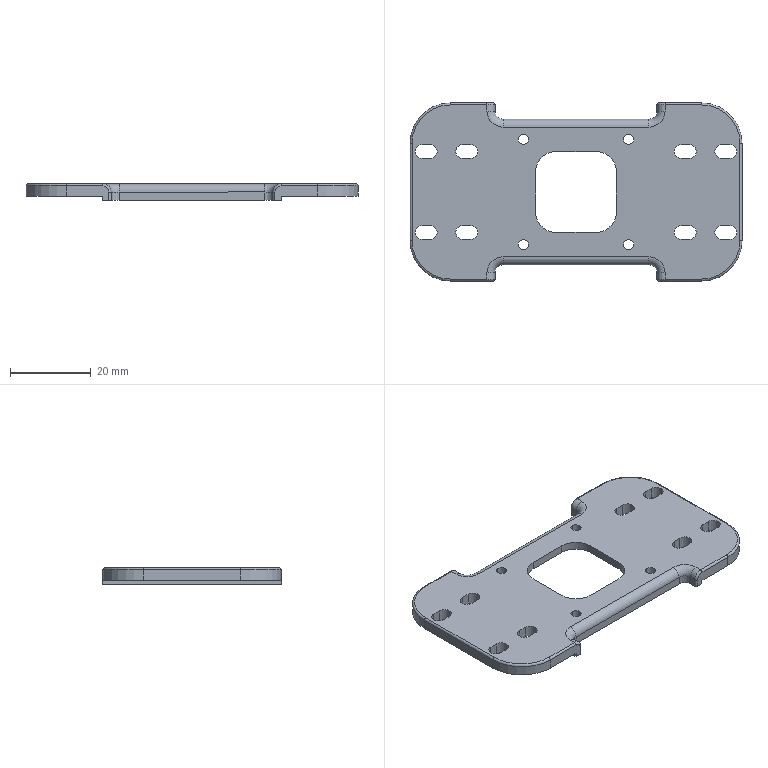NC program | NX | posted with a generic post | part box 82 x 44 x 4 mm
Lines 732 to 1673 of 6362:
(ZLEVEL_PROFILE_COPY_1 , TOOL : D3)
N1432 T16 M6
N1434 G54
N1436 G17 G0 G90 X-19.135 Y22.56 S9500 M3
N1438 G43 Z30. H16
N1440 Z1.214
N1442 G94 G1 Z-0.286 F1000.
N1444 X-19.461 Y22.23
N1446 G3 X-19.537 Y21.94 R0.3
N1448 G2 X-19.47 Y21.5 R1.938 F1200.
N1450 G1 Y20.
N1452 G3 X-18. Y18.53 R1.47
N1454 G1 X-15.874
N1456 G3 X-15.614 Y18.68 R0.3
N1458 G1 X-15.354 Y19.13
N1460 Z1.214
N1462 G0 X-18.813 Y22.683 Z0.929
N1464 G1 Z-0.571 F1000.
N1466 X-19.127 Y22.34
N1468 G3 X-19.191 Y22.047 R0.3
N1470 G2 X-19.1 Y21.5 R1.975 F1200.
N1472 G1 Y20.
N1474 G3 X-18. Y18.9 R1.1
N1476 G1 X-15.569
N1478 G3 X-15.31 Y19.05 R0.3
N1480 G1 X-15.05 Y19.5
N1482 Z0.929
N1484 G0 X-18.644 Y22.827 Z0.643
N1486 G1 Z-0.857 F1000.
N1488 X-18.939 Y22.468
N1490 G3 X-18.987 Y22.171 R0.3
N1492 G2 X-18.859 Y21.5 R1.996 F1200.
N1494 G1 Y20.
N1496 G3 X-18. Y19.141 R0.859
N1498 G1 X-15.358
N1500 G3 X-15.098 Y19.291 R0.3
N1502 G1 X-14.838 Y19.741
N1504 Z0.643
N1506 G0 X-18.512 Y22.893 Z0.357
N1508 G1 Z-1.143 F1000.
N1510 X-18.798 Y22.526
N1512 G3 X-18.84 Y22.229 R0.3
N1514 G2 X-18.693 Y21.5 R2.014 F1200.
N1516 G1 Y20.
N1518 G3 X-18. Y19.307 R0.693
N1520 G1 X-15.23
N1522 G3 X-14.97 Y19.457 R0.3
N1524 G1 X-14.71 Y19.907
N1526 Z0.357
N1528 G0 X-18.421 Y22.93 Z0.071
N1530 G1 Z-1.429 F1000.
N1532 X-18.703 Y22.559
N1534 G3 X-18.741 Y22.262 R0.3
N1536 G2 X-18.583 Y21.5 R2.021 F1200.
N1538 G1 Y20.
N1540 G3 X-18. Y19.417 R0.583
N1542 G1 X-15.149
N1544 G3 X-14.889 Y19.567 R0.3
N1546 G1 X-14.629 Y20.017
N1548 Z0.071
N1550 G0 X-18.396 Y22.989 Z-0.214
N1552 G1 Z-1.714 F1000.
N1554 X-18.668 Y22.611
N1556 G3 X-18.698 Y22.313 R0.3
N1558 G2 X-18.564 Y21.901 R2.015 F1200.
N1560 G1 X-18.521 Y21.5
N1562 Y20.
N1564 G3 X-18. Y19.479 R0.521
N1566 G1 X-15.103
N1568 G3 X-14.843 Y19.629 R0.3
N1570 G1 X-14.583 Y20.079
N1572 Z-0.214
N1574 G0 X-18.361 Y22.977 Z-0.5
N1576 G1 Z-2. F1000.
N1578 X-18.637 Y22.603
N1580 G3 X-18.67 Y22.304 R0.3
N1582 G2 X-18.503 Y21.542 R1.997 F1200.
N1584 G1 X-18.5 Y21.297
N1586 Y20.
N1588 G3 X-18. Y19.5 R0.5
N1590 G1 X-15.098
N1592 G3 X-14.839 Y19.65 R0.3
N1594 G1 X-14.579 Y20.1
N1596 Z-0.5
N1598 G0 X-18.361 Y22.977 Z-0.786
N1600 G1 Z-2.286 F1000.
N1602 X-18.636 Y22.602
N1604 G3 X-18.669 Y22.304 R0.3
N1606 G2 X-18.5 Y21.5 R2. F1200.
N1608 G1 Y20.
N1610 G3 X-18. Y19.5 R0.5
N1612 G1 X-15.083
N1614 G3 X-14.823 Y19.65 R0.3
N1616 G1 X-14.564 Y20.1
N1618 Z-0.786
N1620 G0 X-18.361 Y22.977 Z-1.071
N1622 G1 Z-2.571 F1000.
N1624 X-18.636 Y22.602
N1626 G3 X-18.669 Y22.304 R0.3
N1628 G2 X-18.5 Y21.5 R2. F1200.
N1630 G1 Y20.
N1632 G3 X-18. Y19.5 R0.5
N1634 G1 X-15.083
N1636 G3 X-14.823 Y19.65 R0.3
N1638 G1 X-14.564 Y20.1
N1640 Z-1.071
N1642 G0 X-18.361 Y22.977 Z-1.357
N1644 G1 Z-2.857 F1000.
N1646 X-18.636 Y22.602
N1648 G3 X-18.669 Y22.304 R0.3
N1650 G2 X-18.5 Y21.5 R2. F1200.
N1652 G1 Y20.
N1654 G3 X-18. Y19.5 R0.5
N1656 G1 X-15.083
N1658 G3 X-14.823 Y19.65 R0.3
N1660 G1 X-14.564 Y20.1
N1662 Z-1.357
N1664 G0 X-18.361 Y22.977 Z-1.643
N1666 G1 Z-3.143 F1000.
N1668 X-18.636 Y22.602
N1670 G3 X-18.669 Y22.304 R0.3
N1672 G2 X-18.5 Y21.5 R2. F1200.
N1674 G1 Y20.
N1676 G3 X-18. Y19.5 R0.5
N1678 G1 X-15.083
N1680 G3 X-14.823 Y19.65 R0.3
N1682 G1 X-14.564 Y20.1
N1684 Z-1.643
N1686 G0 X-18.361 Y22.977 Z-1.929
N1688 G1 Z-3.429 F1000.
N1690 X-18.636 Y22.602
N1692 G3 X-18.669 Y22.304 R0.3
N1694 G2 X-18.5 Y21.5 R2. F1200.
N1696 G1 Y20.
N1698 G3 X-18. Y19.5 R0.5
N1700 G1 X-15.083
N1702 G3 X-14.823 Y19.65 R0.3
N1704 G1 X-14.564 Y20.1
N1706 Z-1.929
N1708 G0 X-18.361 Y22.977 Z-2.214
N1710 G1 Z-3.714 F1000.
N1712 X-18.636 Y22.602
N1714 G3 X-18.669 Y22.304 R0.3
N1716 G2 X-18.5 Y21.5 R2. F1200.
N1718 G1 Y20.
N1720 G3 X-18. Y19.5 R0.5
N1722 G1 X-15.083
N1724 G3 X-14.823 Y19.65 R0.3
N1726 G1 X-14.564 Y20.1
N1728 Z-2.214
N1730 G0 X-18.361 Y22.977 Z-2.5
N1732 G1 Z-4. F1000.
N1734 X-18.636 Y22.602
N1736 G3 X-18.669 Y22.304 R0.3
N1738 G2 X-18.5 Y21.5 R2. F1200.
N1740 G1 Y20.
N1742 G3 X-18. Y19.5 R0.5
N1744 G1 X-15.083
N1746 G3 X-14.823 Y19.65 R0.3
N1748 G1 X-14.564 Y20.1
N1750 Z-2.5
N1752 G0 Z30.
N1754 X15.354 Y19.13
N1756 Z1.214
N1758 G1 Z-0.286 F1000.
N1760 X15.614 Y18.68
N1762 G3 X15.874 Y18.53 R0.3
N1764 G1 X18. F1200.
N1766 G3 X19.47 Y20. R1.47
N1768 G1 Y21.5
N1770 G2 X19.538 Y21.94 R1.938
N1772 G3 X19.462 Y22.231 R0.3
N1774 G1 X19.135 Y22.561
N1776 Z1.214
N1778 G0 X15.04 Y19.5 Z0.929
N1780 G1 Z-0.571 F1000.
N1782 X15.3 Y19.05
N1784 G3 X15.56 Y18.9 R0.3
N1786 G1 X18. F1200.
N1788 G3 X19.1 Y20. R1.1
N1790 G1 Y21.5
N1792 G2 X19.192 Y22.047 R1.975
N1794 G3 X19.127 Y22.34 R0.3
N1796 G1 X18.813 Y22.683
N1798 Z0.929
N1800 G0 X14.842 Y19.741 Z0.643
N1802 G1 Z-0.857 F1000.
N1804 X15.102 Y19.291
N1806 G3 X15.362 Y19.141 R0.3
N1808 G1 X18. F1200.
N1810 G3 X18.859 Y20. R0.859
N1812 G1 Y21.5
N1814 G2 X18.986 Y22.168 R1.996
N1816 G3 X18.937 Y22.464 R0.3
N1818 G1 X18.641 Y22.823
N1820 Z0.643
N1822 G0 X14.711 Y19.907 Z0.357
N1824 G1 Z-1.143 F1000.
N1826 X14.971 Y19.457
N1828 G3 X15.231 Y19.307 R0.3
N1830 G1 X18. F1200.
N1832 G3 X18.693 Y20. R0.693
N1834 G1 Y21.5
N1836 G2 X18.838 Y22.225 R2.013
N1838 G3 X18.796 Y22.522 R0.3
N1840 G1 X18.508 Y22.888
N1842 Z0.357
N1844 G0 X14.64 Y20.017 Z0.071
N1846 G1 Z-1.429 F1000.
N1848 X14.9 Y19.567
N1850 G3 X15.16 Y19.417 R0.3
N1852 G1 X18. F1200.
N1854 G3 X18.583 Y20. R0.583
N1856 G1 Y21.5
N1858 G2 X18.742 Y22.265 R2.021
N1860 G3 X18.705 Y22.563 R0.3
N1862 G1 X18.424 Y22.934
N1864 Z0.071
N1866 G0 X14.582 Y20.079 Z-0.214
N1868 G1 Z-1.714 F1000.
N1870 X14.842 Y19.629
N1872 G3 X15.102 Y19.479 R0.3
N1874 G1 X18. F1200.
N1876 G3 X18.521 Y20. R0.521
N1878 G1 Y21.5
N1880 G2 X18.698 Y22.307 R2.16
N1882 G3 X18.663 Y22.605 R0.3
N1884 G1 X18.386 Y22.978
N1886 Z-0.214
N1888 G0 X14.579 Y20.1 Z-0.5
N1890 G1 Z-2. F1000.
N1892 X14.839 Y19.65
N1894 G3 X15.098 Y19.5 R0.3
N1896 G1 X18. F1200.
N1898 G3 X18.5 Y20. R0.499
N1900 G1 X18.501 Y20.073
N1902 Y21.297
N1904 X18.503 Y21.542
N1906 G2 X18.671 Y22.305 R1.998
N1908 G3 X18.638 Y22.603 R0.3
N1910 G1 X18.363 Y22.978
N1912 Z-0.5
N1914 G0 X14.564 Y20.1 Z-0.786
N1916 G1 Z-2.286 F1000.
N1918 X14.823 Y19.65
N1920 G3 X15.083 Y19.5 R0.3
N1922 G1 X18. F1200.
N1924 G3 X18.5 Y20. R0.5
N1926 G1 Y21.5
N1928 X18.507 Y21.649
N1930 X18.506
N1932 G2 X18.669 Y22.304 R2.
N1934 G3 X18.636 Y22.602 R0.3
N1936 G1 X18.361 Y22.977
N1938 Z-0.786
N1940 G0 X14.564 Y20.1 Z-1.071
N1942 G1 Z-2.571 F1000.
N1944 X14.823 Y19.65
N1946 G3 X15.083 Y19.5 R0.3
N1948 G1 X18. F1200.
N1950 G3 X18.5 Y20. R0.5
N1952 G1 Y21.5
N1954 X18.507 Y21.649
N1956 X18.506
N1958 G2 X18.669 Y22.304 R2.
N1960 G3 X18.636 Y22.602 R0.3
N1962 G1 X18.361 Y22.977
N1964 Z-1.071
N1966 G0 X14.564 Y20.1 Z-1.357
N1968 G1 Z-2.857 F1000.
N1970 X14.823 Y19.65
N1972 G3 X15.083 Y19.5 R0.3
N1974 G1 X18. F1200.
N1976 G3 X18.5 Y20. R0.5
N1978 G1 Y21.5
N1980 X18.507 Y21.649
N1982 X18.506
N1984 G2 X18.669 Y22.304 R2.
N1986 G3 X18.636 Y22.602 R0.3
N1988 G1 X18.361 Y22.977
N1990 Z-1.357
N1992 G0 X14.564 Y20.1 Z-1.643
N1994 G1 Z-3.143 F1000.
N1996 X14.823 Y19.65
N1998 G3 X15.083 Y19.5 R0.3
N2000 G1 X18. F1200.
N2002 G3 X18.5 Y20. R0.5
N2004 G1 Y21.5
N2006 X18.507 Y21.649
N2008 X18.506
N2010 G2 X18.669 Y22.304 R2.
N2012 G3 X18.636 Y22.602 R0.3
N2014 G1 X18.361 Y22.977
N2016 Z-1.643
N2018 G0 X14.564 Y20.1 Z-1.929
N2020 G1 Z-3.429 F1000.
N2022 X14.823 Y19.65
N2024 G3 X15.083 Y19.5 R0.3
N2026 G1 X18. F1200.
N2028 G3 X18.5 Y20. R0.5
N2030 G1 Y21.5
N2032 X18.507 Y21.649
N2034 X18.506
N2036 G2 X18.669 Y22.304 R2.
N2038 G3 X18.636 Y22.602 R0.3
N2040 G1 X18.361 Y22.977
N2042 Z-1.929
N2044 G0 X14.564 Y20.1 Z-2.214
N2046 G1 Z-3.714 F1000.
N2048 X14.823 Y19.65
N2050 G3 X15.083 Y19.5 R0.3
N2052 G1 X18. F1200.
N2054 G3 X18.5 Y20. R0.5
N2056 G1 Y21.5
N2058 X18.507 Y21.649
N2060 X18.506
N2062 G2 X18.669 Y22.304 R2.
N2064 G3 X18.636 Y22.602 R0.3
N2066 G1 X18.361 Y22.977
N2068 Z-2.214
N2070 G0 X14.564 Y20.1 Z-2.5
N2072 G1 Z-4. F1000.
N2074 X14.823 Y19.65
N2076 G3 X15.083 Y19.5 R0.3
N2078 G1 X18. F1200.
N2080 G3 X18.5 Y20. R0.5
N2082 G1 Y21.5
N2084 X18.507 Y21.649
N2086 X18.506
N2088 G2 X18.669 Y22.304 R2.
N2090 G3 X18.636 Y22.602 R0.3
N2092 G1 X18.361 Y22.977
N2094 Z-2.5
N2096 G0 Z30.
N2098 X19.135 Y-22.561
N2100 Z1.214
N2102 G1 Z-0.286 F1000.
N2104 X19.462 Y-22.231
N2106 G3 X19.538 Y-21.94 R0.3
N2108 G2 X19.47 Y-21.5 R1.938 F1200.
N2110 G1 Y-20.
N2112 G3 X18. Y-18.53 R1.47
N2114 G1 X15.874
N2116 G3 X15.614 Y-18.68 R0.3
N2118 G1 X15.354 Y-19.13
N2120 Z1.214
N2122 G0 X18.813 Y-22.683 Z0.929
N2124 G1 Z-0.571 F1000.
N2126 X19.127 Y-22.34
N2128 G3 X19.191 Y-22.047 R0.3
N2130 G2 X19.1 Y-21.5 R1.975 F1200.
N2132 G1 Y-20.
N2134 G3 X18. Y-18.9 R1.1
N2136 G1 X15.569
N2138 G3 X15.31 Y-19.05 R0.3
N2140 G1 X15.05 Y-19.5
N2142 Z0.929
N2144 G0 X18.642 Y-22.825 Z0.643
N2146 G1 Z-0.857 F1000.
N2148 X18.937 Y-22.465
N2150 G3 X18.985 Y-22.169 R0.3
N2152 G2 X18.859 Y-21.5 R1.982 F1200.
N2154 G1 Y-20.
N2156 G3 X18. Y-19.141 R0.859
N2158 G1 X15.358
N2160 G3 X15.098 Y-19.291 R0.3
N2162 G1 X14.838 Y-19.741
N2164 Z0.643
N2166 G0 X18.51 Y-22.891 Z0.357
N2168 G1 Z-1.143 F1000.
N2170 X18.797 Y-22.525
N2172 G3 X18.839 Y-22.228 R0.3
N2174 G2 X18.693 Y-21.5 R2.01 F1200.
N2176 G1 Y-20.
N2178 G3 X18. Y-19.307 R0.693
N2180 G1 X15.23
N2182 G3 X14.97 Y-19.457 R0.3
N2184 G1 X14.71 Y-19.907
N2186 Z0.357
N2188 G0 X18.422 Y-22.93 Z0.071
N2190 G1 Z-1.429 F1000.
N2192 X18.703 Y-22.559
N2194 G3 X18.741 Y-22.262 R0.3
N2196 G2 X18.583 Y-21.5 R2.021 F1200.
N2198 G1 Y-20.
N2200 G3 X18. Y-19.417 R0.583
N2202 G1 X15.149
N2204 G3 X14.889 Y-19.567 R0.3
N2206 G1 X14.629 Y-20.017
N2208 Z0.071
N2210 G0 X18.385 Y-22.972 Z-0.214
N2212 G1 Z-1.714 F1000.
N2214 X18.659 Y-22.596
N2216 G3 X18.692 Y-22.298 R0.3
N2218 G2 X18.564 Y-21.901 R2.015 F1200.
N2220 X18.521 Y-21.5 R3.783
N2222 G1 Y-20.
N2224 G3 X18. Y-19.479 R0.521
N2226 G1 X15.103
N2228 G3 X14.843 Y-19.629 R0.3
N2230 G1 X14.583 Y-20.079
N2232 Z-0.214
N2234 G0 X18.358 Y-22.97 Z-0.5
N2236 G1 Z-2. F1000.
N2238 X18.634 Y-22.596
N2240 G3 X18.668 Y-22.298 R0.3
N2242 G2 X18.501 Y-21.5 R2.002 F1200.
N2244 G1 Y-20.
N2246 G3 X18. Y-19.499 R0.501
N2248 G1 X15.091
N2250 G3 X14.831 Y-19.649 R0.3
N2252 G1 X14.572 Y-20.099
N2254 Z-0.5
N2256 G0 X18.361 Y-22.977 Z-0.786
N2258 G1 Z-2.286 F1000.
N2260 X18.636 Y-22.602
N2262 G3 X18.669 Y-22.304 R0.3
N2264 G2 X18.5 Y-21.5 R2. F1200.
N2266 G1 Y-20.
N2268 G3 X18. Y-19.5 R0.5
N2270 G1 X15.083
N2272 G3 X14.823 Y-19.65 R0.3
N2274 G1 X14.564 Y-20.1
N2276 Z-0.786
N2278 G0 X18.361 Y-22.977 Z-1.071
N2280 G1 Z-2.571 F1000.
N2282 X18.636 Y-22.602
N2284 G3 X18.669 Y-22.304 R0.3
N2286 G2 X18.5 Y-21.5 R2. F1200.
N2288 G1 Y-20.
N2290 G3 X18. Y-19.5 R0.5
N2292 G1 X15.083
N2294 G3 X14.823 Y-19.65 R0.3
N2296 G1 X14.564 Y-20.1
N2298 Z-1.071
N2300 G0 X18.361 Y-22.977 Z-1.357
N2302 G1 Z-2.857 F1000.
N2304 X18.636 Y-22.602
N2306 G3 X18.669 Y-22.304 R0.3
N2308 G2 X18.5 Y-21.5 R2. F1200.
N2310 G1 Y-20.
N2312 G3 X18. Y-19.5 R0.5
N2314 G1 X15.083
N2316 G3 X14.823 Y-19.65 R0.3
N2318 G1 X14.564 Y-20.1
N2320 Z-1.357
N2322 G0 X18.361 Y-22.977 Z-1.643
N2324 G1 Z-3.143 F1000.
N2326 X18.636 Y-22.602
N2328 G3 X18.669 Y-22.304 R0.3
N2330 G2 X18.5 Y-21.5 R2. F1200.
N2332 G1 Y-20.
N2334 G3 X18. Y-19.5 R0.5
N2336 G1 X15.083
N2338 G3 X14.823 Y-19.65 R0.3
N2340 G1 X14.564 Y-20.1
N2342 Z-1.643
N2344 G0 X18.361 Y-22.977 Z-1.929
N2346 G1 Z-3.429 F1000.
N2348 X18.636 Y-22.602
N2350 G3 X18.669 Y-22.304 R0.3
N2352 G2 X18.5 Y-21.5 R2. F1200.
N2354 G1 Y-20.
N2356 G3 X18. Y-19.5 R0.5
N2358 G1 X15.083
N2360 G3 X14.823 Y-19.65 R0.3
N2362 G1 X14.564 Y-20.1
N2364 Z-1.929
N2366 G0 X18.361 Y-22.977 Z-2.214
N2368 G1 Z-3.714 F1000.
N2370 X18.636 Y-22.602
N2372 G3 X18.669 Y-22.304 R0.3
N2374 G2 X18.5 Y-21.5 R2. F1200.
N2376 G1 Y-20.
N2378 G3 X18. Y-19.5 R0.5
N2380 G1 X15.083
N2382 G3 X14.823 Y-19.65 R0.3
N2384 G1 X14.564 Y-20.1
N2386 Z-2.214
N2388 G0 X18.361 Y-22.977 Z-2.5
N2390 G1 Z-4. F1000.
N2392 X18.636 Y-22.602
N2394 G3 X18.669 Y-22.304 R0.3
N2396 G2 X18.5 Y-21.5 R2. F1200.
N2398 G1 Y-20.
N2400 G3 X18. Y-19.5 R0.5
N2402 G1 X15.083
N2404 G3 X14.823 Y-19.65 R0.3
N2406 G1 X14.564 Y-20.1
N2408 Z-2.5
N2410 G0 Z30.
N2412 X-15.354 Y-19.13
N2414 Z1.214
N2416 G1 Z-0.286 F1000.
N2418 X-15.614 Y-18.68
N2420 G3 X-15.874 Y-18.53 R0.3
N2422 G1 X-18. F1200.
N2424 G3 X-19.47 Y-20. R1.47
N2426 G1 Y-21.5
N2428 G2 X-19.537 Y-21.94 R1.938
N2430 G3 X-19.462 Y-22.23 R0.3
N2432 G1 X-19.135 Y-22.561
N2434 Z1.214
N2436 G0 X-15.04 Y-19.5 Z0.929
N2438 G1 Z-0.571 F1000.
N2440 X-15.3 Y-19.05
N2442 G3 X-15.56 Y-18.9 R0.3
N2444 G1 X-18. F1200.
N2446 G3 X-19.1 Y-20. R1.1
N2448 G1 Y-21.5
N2450 G2 X-19.192 Y-22.047 R1.975
N2452 G3 X-19.127 Y-22.34 R0.3
N2454 G1 X-18.813 Y-22.683
N2456 Z0.929
N2458 G0 X-14.842 Y-19.741 Z0.643
N2460 G1 Z-0.857 F1000.
N2462 X-15.102 Y-19.291
N2464 G3 X-15.362 Y-19.141 R0.3
N2466 G1 X-18. F1200.
N2468 G3 X-18.859 Y-20. R0.859
N2470 G1 Y-21.5
N2472 G2 X-18.986 Y-22.168 R1.996
N2474 G3 X-18.937 Y-22.464 R0.3
N2476 G1 X-18.641 Y-22.823
N2478 Z0.643
N2480 G0 X-14.711 Y-19.907 Z0.357
N2482 G1 Z-1.143 F1000.
N2484 X-14.971 Y-19.457
N2486 G3 X-15.231 Y-19.307 R0.3
N2488 G1 X-18. F1200.
N2490 G3 X-18.693 Y-20. R0.693
N2492 G1 Y-21.5
N2494 G2 X-18.838 Y-22.225 R2.013
N2496 G3 X-18.796 Y-22.522 R0.3
N2498 G1 X-18.508 Y-22.888
N2500 Z0.357
N2502 G0 X-14.64 Y-20.017 Z0.071
N2504 G1 Z-1.429 F1000.
N2506 X-14.9 Y-19.567
N2508 G3 X-15.16 Y-19.417 R0.3
N2510 G1 X-18. F1200.
N2512 G3 X-18.583 Y-20. R0.583
N2514 G1 Y-21.5
N2516 G2 X-18.742 Y-22.265 R2.021
N2518 G3 X-18.705 Y-22.563 R0.3
N2520 G1 X-18.424 Y-22.934
N2522 Z0.071
N2524 G0 X-14.583 Y-20.079 Z-0.214
N2526 G1 Z-1.714 F1000.
N2528 X-14.842 Y-19.629
N2530 G3 X-15.102 Y-19.479 R0.3
N2532 G1 X-18. F1200.
N2534 G3 X-18.521 Y-20. R0.521
N2536 G1 Y-21.5
N2538 G2 X-18.696 Y-22.304 R2.152
N2540 G3 X-18.662 Y-22.602 R0.3
N2542 G1 X-18.385 Y-22.975
N2544 Z-0.214
N2546 G0 X-14.569 Y-20.099 Z-0.5
N2548 G1 Z-2. F1000.
N2550 X-14.829 Y-19.649
N2552 G3 X-15.089 Y-19.499 R0.3
N2554 G1 X-18. F1200.
N2556 G3 X-18.501 Y-20. R0.503
N2558 G1 Y-21.5
N2560 X-18.503 Y-21.542
N2562 G2 X-18.678 Y-22.32 R1.999
N2564 G3 X-18.648 Y-22.619 R0.3
N2566 G1 X-18.375 Y-22.996
N2568 Z-0.5
N2570 G0 X-14.584 Y-20.1 Z-0.786
N2572 G1 Z-2.286 F1000.
N2574 X-14.844 Y-19.65
N2576 G3 X-15.104 Y-19.5 R0.3
N2578 G1 X-18. F1200.
N2580 G3 X-18.5 Y-20. R0.5
N2582 G1 Y-21.5
N2584 X-18.509 Y-21.664
N2586 X-18.507 Y-21.665
N2588 G2 X-18.668 Y-22.303 R2.
N2590 G3 X-18.635 Y-22.602 R0.3
N2592 G1 X-18.36 Y-22.977
N2594 Z-0.786
N2596 G0 X-14.584 Y-20.1 Z-1.071
N2598 G1 Z-2.571 F1000.
N2600 X-14.844 Y-19.65
N2602 G3 X-15.104 Y-19.5 R0.3
N2604 G1 X-18. F1200.
N2606 G3 X-18.5 Y-20. R0.5
N2608 G1 Y-21.5
N2610 X-18.509 Y-21.664
N2612 X-18.507 Y-21.665
N2614 G2 X-18.668 Y-22.303 R2.
N2616 G3 X-18.635 Y-22.602 R0.3
N2618 G1 X-18.36 Y-22.977
N2620 Z-1.071
N2622 G0 X-14.584 Y-20.1 Z-1.357
N2624 G1 Z-2.857 F1000.
N2626 X-14.844 Y-19.65
N2628 G3 X-15.103 Y-19.5 R0.3
N2630 G1 X-18. F1200.
N2632 G3 X-18.5 Y-20. R0.5
N2634 G1 Y-21.5
N2636 X-18.509 Y-21.664
N2638 X-18.507 Y-21.665
N2640 G2 X-18.668 Y-22.303 R2.
N2642 G3 X-18.636 Y-22.602 R0.3
N2644 G1 X-18.36 Y-22.977
N2646 Z-1.357
N2648 G0 X-14.584 Y-20.1 Z-1.643
N2650 G1 Z-3.143 F1000.
N2652 X-14.843 Y-19.65
N2654 G3 X-15.103 Y-19.5 R0.3
N2656 G1 X-18. F1200.
N2658 G3 X-18.5 Y-20. R0.5
N2660 G1 Y-21.5
N2662 X-18.509 Y-21.664
N2664 X-18.507 Y-21.665
N2666 G2 X-18.668 Y-22.303 R2.
N2668 G3 X-18.636 Y-22.602 R0.3
N2670 G1 X-18.36 Y-22.977
N2672 Z-1.643
N2674 G0 X-14.583 Y-20.1 Z-1.929
N2676 G1 Z-3.429 F1000.
N2678 X-14.843 Y-19.65
N2680 G3 X-15.103 Y-19.5 R0.3
N2682 G1 X-18. F1200.
N2684 G3 X-18.5 Y-20. R0.5
N2686 G1 Y-21.5
N2688 X-18.509 Y-21.664
N2690 X-18.507 Y-21.665
N2692 G2 X-18.668 Y-22.303 R2.
N2694 G3 X-18.636 Y-22.602 R0.3
N2696 G1 X-18.36 Y-22.977
N2698 Z-1.929
N2700 G0 X-14.583 Y-20.1 Z-2.214
N2702 G1 Z-3.714 F1000.
N2704 X-14.843 Y-19.65
N2706 G3 X-15.103 Y-19.5 R0.3
N2708 G1 X-18. F1200.
N2710 G3 X-18.5 Y-20. R0.5
N2712 G1 Y-21.5
N2714 X-18.509 Y-21.664
N2716 X-18.507 Y-21.665
N2718 G2 X-18.669 Y-22.303 R2.
N2720 G3 X-18.636 Y-22.602 R0.3
N2722 G1 X-18.36 Y-22.977
N2724 Z-2.214
N2726 G0 X-14.583 Y-20.1 Z-2.5
N2728 G1 Z-4. F1000.
N2730 X-14.843 Y-19.65
N2732 G3 X-15.103 Y-19.5 R0.3
N2734 G1 X-18. F1200.
N2736 G3 X-18.5 Y-20. R0.5
N2738 G1 Y-21.5
N2740 X-18.509 Y-21.664
N2742 X-18.507 Y-21.665
N2744 G2 X-18.669 Y-22.304 R2.
N2746 G3 X-18.636 Y-22.602 R0.3
N2748 G1 X-18.36 Y-22.977
N2750 Z-2.5
N2752 G0 Z30.
(ZLEVEL_PROFILE_COPY_2 , TOOL : D3)
N2754 X-27.684 Y10.2 S9509
N2756 Z1.
N2758 G1 X-28.064 Z0.98 F1000.
N2760 X-28.073 Y10.197
N2762 X-28.174 Y10.118 Z0.973
N2764 X-28.21 Y10.001 Z0.966
N2766 X-28.174 Y9.883 Z0.96
N2768 X-28.074 Y9.803 Z0.953
N2770 X-28.064 Y9.8
N2772 X-25.971 Z0.843
N2774 X-25.882 Y9.826 Z0.838
N2776 X-25.801 Y9.933 Z0.831
N2778 Y10.067 Z0.824
N2780 X-25.877 Y10.17 Z0.817
N2782 X-25.936 Y10.2 Z0.814
N2784 X-28.064 Z0.702
N2786 X-28.073 Y10.197
N2788 X-28.174 Y10.118 Z0.695
N2790 X-28.21 Y10.001 Z0.689
N2792 X-28.174 Y9.883 Z0.682
N2794 X-28.074 Y9.803 Z0.676
N2796 X-28.064 Y9.8 Z0.675
N2798 X-25.971 Z0.565
N2800 X-25.882 Y9.826 Z0.561
N2802 X-25.801 Y9.933 Z0.554
N2804 Y10.067 Z0.547
N2806 X-25.877 Y10.17 Z0.54
N2808 X-25.936 Y10.2 Z0.536
N2810 X-28.064 Z0.425
N2812 X-28.073 Y10.197 Z0.424
N2814 X-28.174 Y10.118 Z0.418
N2816 X-28.21 Y10.001 Z0.411
N2818 X-28.174 Y9.883 Z0.405
N2820 X-28.074 Y9.803 Z0.398
N2822 X-28.064 Y9.8 Z0.397
N2824 X-25.971 Z0.288
N2826 X-25.882 Y9.826 Z0.283
N2828 X-25.801 Y9.933 Z0.276
N2830 Y10.067 Z0.269
N2832 X-25.877 Y10.17 Z0.262
N2834 X-25.936 Y10.2 Z0.259
N2836 X-28.064 Z0.147
N2838 X-28.073 Y10.197
N2840 X-28.174 Y10.118 Z0.14
N2842 X-28.21 Y10.001 Z0.133
N2844 X-28.174 Y9.883 Z0.127
N2846 X-28.074 Y9.803 Z0.12
N2848 X-28.064 Y9.8
N2850 X-25.971 Z0.01
N2852 X-25.882 Y9.826 Z0.005
N2854 X-25.801 Y9.933 Z-0.002
N2856 Y10.067 Z-0.009
N2858 X-25.877 Y10.17 Z-0.015
N2860 X-25.936 Y10.2 Z-0.019
N2862 X-28.064 Z-0.131
N2864 X-28.073 Y10.197
N2866 X-28.174 Y10.118 Z-0.138
N2868 X-28.21 Y10.001 Z-0.144
N2870 X-28.174 Y9.883 Z-0.151
N2872 X-28.074 Y9.803 Z-0.157
N2874 X-28.064 Y9.8 Z-0.158
N2876 X-25.971 Z-0.268
N2878 X-25.882 Y9.826 Z-0.272
N2880 X-25.801 Y9.933 Z-0.279
N2882 Y10.067 Z-0.286
N2884 X-25.877 Y10.17 Z-0.293
N2886 X-25.936 Y10.2 Z-0.297
N2888 X-26. Z-0.3
N2890 X-28. F1350.
N2892 G3 X-28.2 Y10. R0.2
N2894 X-28. Y9.8 R0.2
N2896 G1 X-26.
N2898 G3 X-25.8 Y10. R0.2
N2900 X-26. Y10.2 R0.2
N2902 G1 X-28. Z-0.414
N2904 X-28.044 Y10.195 Z-0.417
N2906 X-28.065 Y10.189 Z-0.418
N2908 X-28.106 Y10.17 Z-0.421
N2910 X-28.123 Y10.157 Z-0.422
N2912 X-28.173 Y10.101 Z-0.426
N2914 X-28.191 Y10.06 Z-0.429
N2916 X-28.2 Y9.99 Z-0.433
N2918 X-28.191 Y9.941 Z-0.436
N2920 X-28.163 Y9.885 Z-0.439
N2922 X-28.124 Y9.843 Z-0.442
N2924 X-28.095 Y9.824 Z-0.444
N2926 X-28.066 Y9.811 Z-0.446
N2928 X-28.04 Y9.804 Z-0.448
N2930 X-28. Y9.8 Z-0.45
N2932 X-26. Z-0.564
N2934 X-25.959 Y9.804 Z-0.567
N2936 X-25.944 Y9.808 Z-0.568
N2938 X-25.889 Y9.834 Z-0.571
N2940 X-25.862 Y9.856 Z-0.573
N2942 X-25.827 Y9.9 Z-0.576
N2944 X-25.811 Y9.936 Z-0.578
N2946 X-25.8 Y9.991 Z-0.582
N2948 X-25.802 Y10.03 Z-0.584
N2950 X-25.818 Y10.084 Z-0.587
N2952 X-25.839 Y10.118 Z-0.589
N2954 X-25.877 Y10.157 Z-0.592
N2956 X-25.91 Y10.178 Z-0.595
N2958 X-25.954 Y10.195 Z-0.597
N2960 X-26. Y10.2 Z-0.6
N2962 X-28. Z-0.714
N2964 X-28.044 Y10.195 Z-0.717
N2966 X-28.065 Y10.189 Z-0.718
N2968 X-28.106 Y10.17 Z-0.721
N2970 X-28.123 Y10.157 Z-0.722
N2972 X-28.173 Y10.101 Z-0.726
N2974 X-28.191 Y10.06 Z-0.729
N2976 X-28.2 Y9.99 Z-0.733
N2978 X-28.191 Y9.941 Z-0.736
N2980 X-28.163 Y9.885 Z-0.739
N2982 X-28.124 Y9.843 Z-0.742
N2984 X-28.095 Y9.824 Z-0.744
N2986 X-28.066 Y9.811 Z-0.746
N2988 X-28.04 Y9.804 Z-0.748
N2990 X-28. Y9.8 Z-0.75
N2992 X-26. Z-0.864
N2994 X-25.959 Y9.804 Z-0.867
N2996 X-25.944 Y9.808 Z-0.868
N2998 X-25.889 Y9.834 Z-0.871
N3000 X-25.862 Y9.856 Z-0.873
N3002 X-25.827 Y9.9 Z-0.876
N3004 X-25.811 Y9.936 Z-0.878
N3006 X-25.8 Y9.991 Z-0.882
N3008 X-25.802 Y10.03 Z-0.884
N3010 X-25.818 Y10.084 Z-0.887
N3012 X-25.839 Y10.118 Z-0.889
N3014 X-25.877 Y10.157 Z-0.892
N3016 X-25.91 Y10.178 Z-0.895
N3018 X-25.954 Y10.195 Z-0.897
N3020 X-26. Y10.2 Z-0.9
N3022 X-28. Z-1.014
N3024 X-28.044 Y10.195 Z-1.017
N3026 X-28.065 Y10.189 Z-1.018
N3028 X-28.106 Y10.17 Z-1.021
N3030 X-28.123 Y10.157 Z-1.022
N3032 X-28.173 Y10.101 Z-1.026
N3034 X-28.191 Y10.06 Z-1.029
N3036 X-28.2 Y9.99 Z-1.033
N3038 X-28.191 Y9.941 Z-1.036
N3040 X-28.163 Y9.885 Z-1.039
N3042 X-28.124 Y9.843 Z-1.042
N3044 X-28.095 Y9.824 Z-1.044
N3046 X-28.066 Y9.811 Z-1.046
N3048 X-28.04 Y9.804 Z-1.048
N3050 X-28. Y9.8 Z-1.05
N3052 X-26. Z-1.164
N3054 X-25.959 Y9.804 Z-1.167
N3056 X-25.944 Y9.808 Z-1.168
N3058 X-25.889 Y9.834 Z-1.171
N3060 X-25.862 Y9.856 Z-1.173
N3062 X-25.827 Y9.9 Z-1.176
N3064 X-25.811 Y9.936 Z-1.178
N3066 X-25.8 Y9.991 Z-1.182
N3068 X-25.802 Y10.03 Z-1.184
N3070 X-25.818 Y10.084 Z-1.187
N3072 X-25.839 Y10.118 Z-1.189
N3074 X-25.877 Y10.157 Z-1.192
N3076 X-25.91 Y10.178 Z-1.195
N3078 X-25.954 Y10.195 Z-1.197
N3080 X-26. Y10.2 Z-1.2
N3082 X-28. Z-1.314
N3084 X-28.044 Y10.195 Z-1.317
N3086 X-28.065 Y10.189 Z-1.318
N3088 X-28.106 Y10.17 Z-1.321
N3090 X-28.123 Y10.157 Z-1.322
N3092 X-28.173 Y10.101 Z-1.326
N3094 X-28.191 Y10.06 Z-1.329
N3096 X-28.2 Y9.99 Z-1.333
N3098 X-28.191 Y9.941 Z-1.336
N3100 X-28.163 Y9.885 Z-1.339
N3102 X-28.124 Y9.843 Z-1.342
N3104 X-28.095 Y9.824 Z-1.344
N3106 X-28.066 Y9.811 Z-1.346
N3108 X-28.04 Y9.804 Z-1.348
N3110 X-28. Y9.8 Z-1.35
N3112 X-26. Z-1.464
N3114 X-25.959 Y9.804 Z-1.467
N3116 X-25.944 Y9.808 Z-1.468
N3118 X-25.889 Y9.834 Z-1.471
N3120 X-25.862 Y9.856 Z-1.473
N3122 X-25.827 Y9.9 Z-1.476
N3124 X-25.811 Y9.936 Z-1.478
N3126 X-25.8 Y9.991 Z-1.482
N3128 X-25.802 Y10.03 Z-1.484
N3130 X-25.818 Y10.084 Z-1.487
N3132 X-25.839 Y10.118 Z-1.489
N3134 X-25.877 Y10.157 Z-1.492
N3136 X-25.91 Y10.178 Z-1.495
N3138 X-25.954 Y10.195 Z-1.497
N3140 X-26. Y10.2 Z-1.5
N3142 X-28. Z-1.614
N3144 X-28.044 Y10.195 Z-1.617
N3146 X-28.065 Y10.189 Z-1.618
N3148 X-28.106 Y10.17 Z-1.621
N3150 X-28.123 Y10.157 Z-1.622
N3152 X-28.173 Y10.101 Z-1.626
N3154 X-28.191 Y10.06 Z-1.629
N3156 X-28.2 Y9.99 Z-1.633
N3158 X-28.191 Y9.941 Z-1.636
N3160 X-28.163 Y9.885 Z-1.639
N3162 X-28.124 Y9.843 Z-1.642
N3164 X-28.095 Y9.824 Z-1.644
N3166 X-28.066 Y9.811 Z-1.646
N3168 X-28.04 Y9.804 Z-1.648
N3170 X-28. Y9.8 Z-1.65
N3172 X-26. Z-1.764
N3174 X-25.959 Y9.804 Z-1.767
N3176 X-25.944 Y9.808 Z-1.768
N3178 X-25.889 Y9.834 Z-1.771
N3180 X-25.862 Y9.856 Z-1.773
N3182 X-25.827 Y9.9 Z-1.776
N3184 X-25.811 Y9.936 Z-1.778
N3186 X-25.8 Y9.991 Z-1.782
N3188 X-25.802 Y10.03 Z-1.784
N3190 X-25.818 Y10.084 Z-1.787
N3192 X-25.839 Y10.118 Z-1.789
N3194 X-25.877 Y10.157 Z-1.792
N3196 X-25.91 Y10.178 Z-1.795
N3198 X-25.954 Y10.195 Z-1.797
N3200 X-26. Y10.2 Z-1.8
N3202 X-28. Z-1.914
N3204 X-28.044 Y10.195 Z-1.917
N3206 X-28.065 Y10.189 Z-1.918
N3208 X-28.106 Y10.17 Z-1.921
N3210 X-28.123 Y10.157 Z-1.922
N3212 X-28.173 Y10.101 Z-1.926
N3214 X-28.191 Y10.06 Z-1.929
N3216 X-28.2 Y9.99 Z-1.933
N3218 X-28.191 Y9.941 Z-1.936
N3220 X-28.163 Y9.885 Z-1.939
N3222 X-28.124 Y9.843 Z-1.942
N3224 X-28.095 Y9.824 Z-1.944
N3226 X-28.066 Y9.811 Z-1.946
N3228 X-28.04 Y9.804 Z-1.948
N3230 X-28. Y9.8 Z-1.95
N3232 X-26. Z-2.064
N3234 X-25.959 Y9.804 Z-2.067
N3236 X-25.944 Y9.808 Z-2.068
N3238 X-25.889 Y9.834 Z-2.071
N3240 X-25.862 Y9.856 Z-2.073
N3242 X-25.827 Y9.9 Z-2.076
N3244 X-25.811 Y9.936 Z-2.078
N3246 X-25.8 Y9.991 Z-2.082
N3248 X-25.802 Y10.03 Z-2.084
N3250 X-25.818 Y10.084 Z-2.087
N3252 X-25.839 Y10.118 Z-2.089
N3254 X-25.877 Y10.157 Z-2.092
N3256 X-25.91 Y10.178 Z-2.095
N3258 X-25.954 Y10.195 Z-2.097
N3260 X-26. Y10.2 Z-2.1
N3262 X-28. Z-2.214
N3264 X-28.044 Y10.195 Z-2.217
N3266 X-28.065 Y10.189 Z-2.218
N3268 X-28.106 Y10.17 Z-2.221
N3270 X-28.123 Y10.157 Z-2.222
N3272 X-28.173 Y10.101 Z-2.226
N3274 X-28.191 Y10.06 Z-2.229
N3276 X-28.2 Y9.99 Z-2.233
N3278 X-28.191 Y9.941 Z-2.236
N3280 X-28.163 Y9.885 Z-2.239
N3282 X-28.124 Y9.843 Z-2.242
N3284 X-28.095 Y9.824 Z-2.244
N3286 X-28.066 Y9.811 Z-2.246
N3288 X-28.04 Y9.804 Z-2.248
N3290 X-28. Y9.8 Z-2.25
N3292 X-26. Z-2.364
N3294 X-25.959 Y9.804 Z-2.367
N3296 X-25.944 Y9.808 Z-2.368
N3298 X-25.889 Y9.834 Z-2.371
N3300 X-25.862 Y9.856 Z-2.373
N3302 X-25.827 Y9.9 Z-2.376